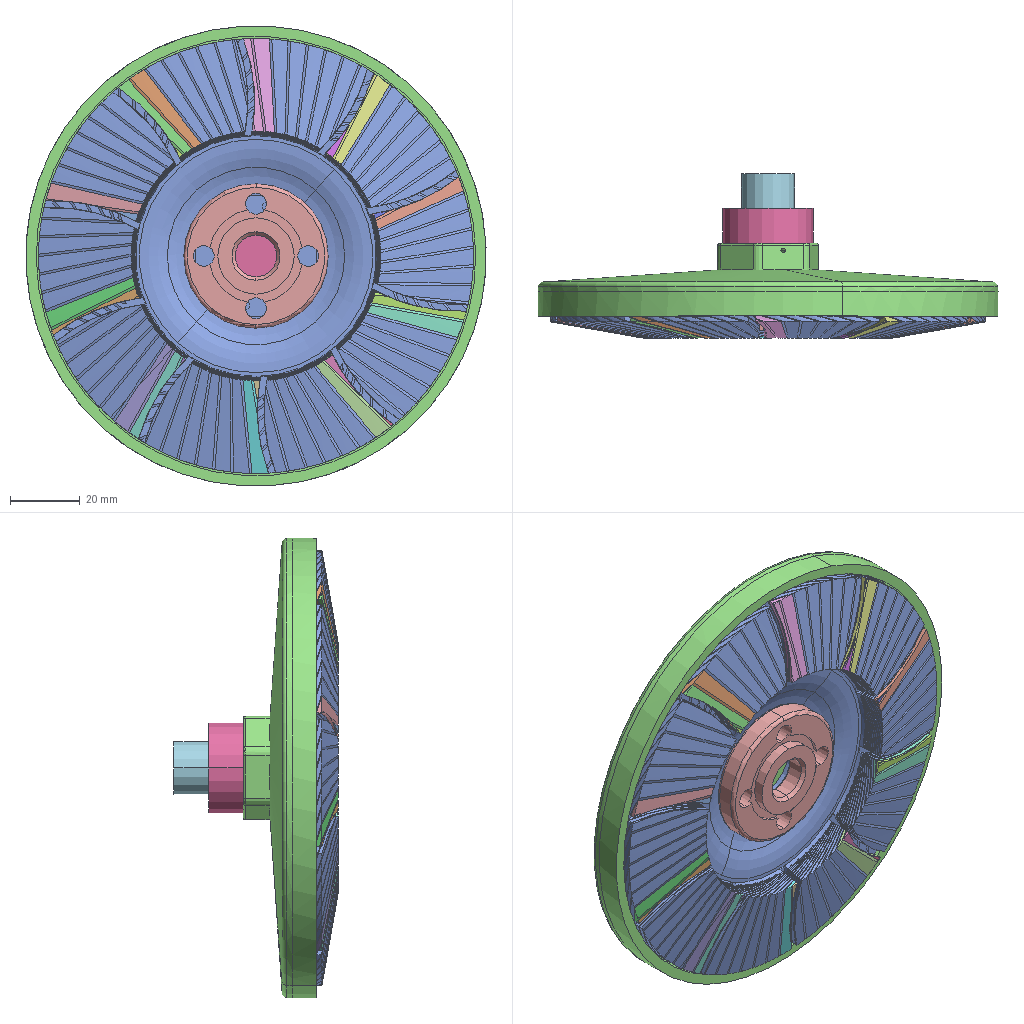Assembly | SolidWorks | 6 different items | 6 placed | box 132 x 47 x 132 mm
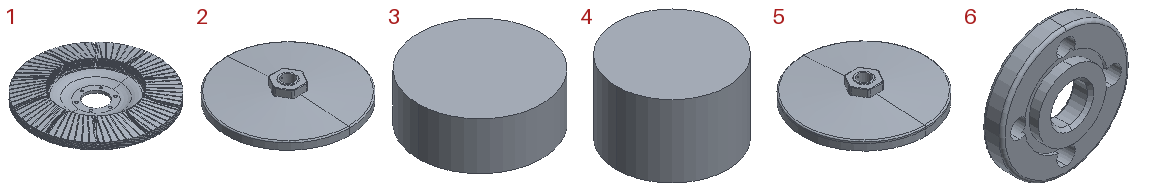Parts list (item | quantity | size | volume | features):
1 | x1 | 125 x 125 x 13.257 mm | 65573 mm3 | features BaseBody 1, CutThin 1
2 | x1 | 49.005 x 49.005 x 7.489 mm | 6259 mm3 | features ICE 5, Fillet 3, BossThin 2, CirPattern 1, CutThin 1, Extrusion 1, Revolution 1
3 | x1 | 25.927 x 25.927 x 10 mm | 5280 mm3 | features Extrusion 1
4 | x1 | 15.395 x 15.395 x 10 mm | 1861 mm3 | features Extrusion 1
5 | x1 | 132.316 x 132.316 x 21.819 mm | 70046 mm3 | features Fillet 3, ICE 3, BossThin 2, Extrusion 1, Revolution 1, Scale 1
6 | x1 | 41.5 x 8.5 x 41.5 mm | 6920 mm3 | features BaseBody 1
Mates (type | each side: item.copy, entity, surface, feature):
Parallel | 1.1 face plane Import1 | 5.1 face plane Revolve1
Concentric | 6.1 face cylinder Import1 | 5.1 face cylinder Boss-Extrude
Coincident | 1.1 face plane Import1 | 5.1 face plane Revolve1